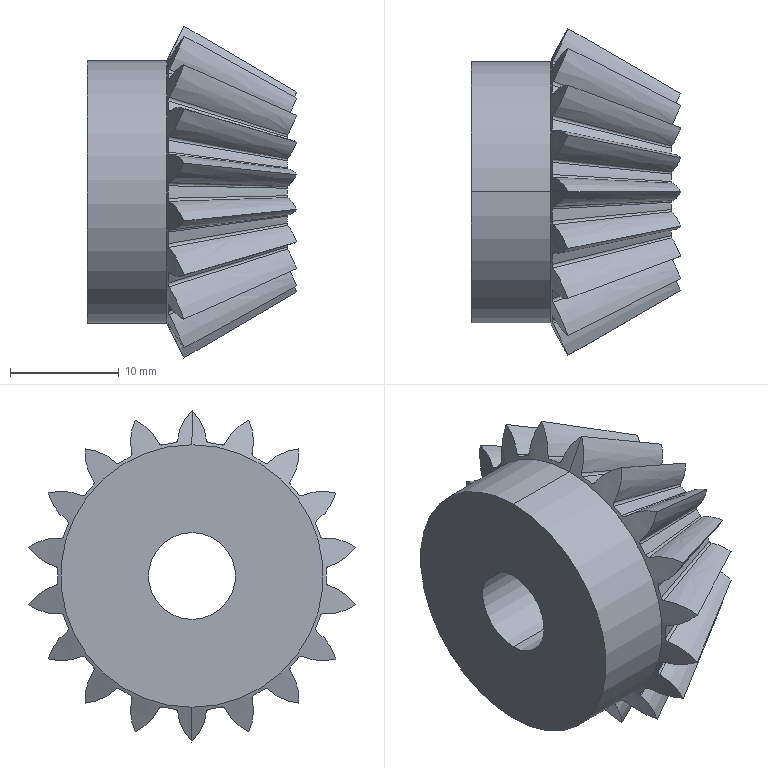Part | SolidWorks | features CirPattern 2, Cut 2, BlendCut 1, Boss 1, Revolution 1 | 1 solid | 100 faces | box 19.27 x 30.102 x 30.566 mm | volume 6755 mm3 | spline 90 | cylinder 4 | cone 4 | plane 2 | commonest cylinder face diameters 8 x2 24.17 x2